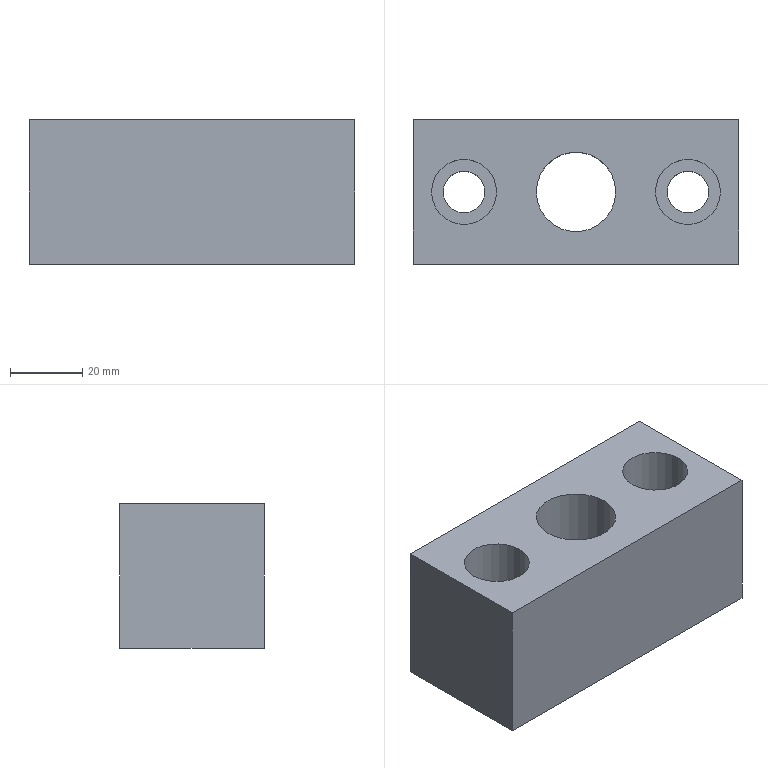Part | STEP file | lll_id4838_x_t | 1 solid | 15 faces | box 90 x 40 x 40 mm | volume 115299 mm3 | plane 9 | cylinder 6 | commonest cylinder face diameters 11.509 x2 18.008 x2 22 x1 30 x1
STEP:
#1=CARTESIAN_POINT('',(2582.,20.,-80.));
#2=VERTEX_POINT('',#1);
#3=CARTESIAN_POINT('',(2582.,-20.,-80.));
#4=VERTEX_POINT('',#3);
#5=CARTESIAN_POINT('',(2582.,10.,-80.));
#6=DIRECTION('',(0.,-1.,0.));
#7=VECTOR('',#6,1.);
#8=LINE('',#5,#7);
#9=EDGE_CURVE('',#2,#4,#8,.T.);
#10=ORIENTED_EDGE('',*,*,#9,.F.);
#11=CARTESIAN_POINT('',(2672.,20.,-80.));
#12=VERTEX_POINT('',#11);
#13=CARTESIAN_POINT('',(2632.,20.,-80.));
#14=DIRECTION('',(-1.,0.,0.));
#15=VECTOR('',#14,1.);
#16=LINE('',#13,#15);
#17=EDGE_CURVE('',#12,#2,#16,.T.);
#18=ORIENTED_EDGE('',*,*,#17,.F.);
#19=CARTESIAN_POINT('',(2672.,-20.,-80.));
#20=VERTEX_POINT('',#19);
#21=CARTESIAN_POINT('',(2672.,10.,-80.));
#22=DIRECTION('',(0.,1.,0.));
#23=VECTOR('',#22,1.);
#24=LINE('',#21,#23);
#25=EDGE_CURVE('',#20,#12,#24,.T.);
#26=ORIENTED_EDGE('',*,*,#25,.F.);
#27=CARTESIAN_POINT('',(2632.,-20.,-80.));
#28=DIRECTION('',(1.,0.,0.));
#29=VECTOR('',#28,1.);
#30=LINE('',#27,#29);
#31=EDGE_CURVE('',#4,#20,#30,.T.);
#32=ORIENTED_EDGE('',*,*,#31,.F.);
#33=EDGE_LOOP('',(#10,#18,#26,#32));
#34=FACE_BOUND('',#33,.T.);
#35=CARTESIAN_POINT('',(2663.755,0.00007613,-80.));
#36=VERTEX_POINT('',#35);
#37=CARTESIAN_POINT('',(2658.,0.00007613,-80.));
#38=DIRECTION('',(0.,0.,-1.));
#39=DIRECTION('',(1.,0.,0.));
#40=AXIS2_PLACEMENT_3D('',#37,#38,#39);
#41=CIRCLE('',#40,5.755);
#42=EDGE_CURVE('',#36,#36,#41,.T.);
#43=ORIENTED_EDGE('',*,*,#42,.F.);
#44=EDGE_LOOP('',(#43));
#45=FACE_BOUND('',#44,.T.);
#46=CARTESIAN_POINT('',(2601.755,0.00007613,-80.));
#47=VERTEX_POINT('',#46);
#48=CARTESIAN_POINT('',(2596.,0.00007613,-80.));
#49=DIRECTION('',(0.,0.,-1.));
#50=DIRECTION('',(1.,0.,0.));
#51=AXIS2_PLACEMENT_3D('',#48,#49,#50);
#52=CIRCLE('',#51,5.755);
#53=EDGE_CURVE('',#47,#47,#52,.T.);
#54=ORIENTED_EDGE('',*,*,#53,.F.);
#55=EDGE_LOOP('',(#54));
#56=FACE_BOUND('',#55,.T.);
#57=CARTESIAN_POINT('',(2612.,0.00007613,-80.));
#58=VERTEX_POINT('',#57);
#59=CARTESIAN_POINT('',(2627.,0.00007613,-80.));
#60=DIRECTION('',(0.,0.,1.));
#61=DIRECTION('',(-1.,0.,0.));
#62=AXIS2_PLACEMENT_3D('',#59,#60,#61);
#63=CIRCLE('',#62,15.);
#64=EDGE_CURVE('',#58,#58,#63,.T.);
#65=ORIENTED_EDGE('',*,*,#64,.T.);
#66=EDGE_LOOP('',(#65));
#67=FACE_BOUND('',#66,.T.);
#68=CARTESIAN_POINT('',(2632.,10.,-80.));
#69=DIRECTION('',(0.,0.,-1.));
#70=DIRECTION('',(1.,0.,0.));
#71=AXIS2_PLACEMENT_3D('',#68,#69,#70);
#72=PLANE('',#71);
#73=ADVANCED_FACE('',(#34,#45,#56,#67),#72,.T.);
#74=CARTESIAN_POINT('',(2638.,0.00007613,-40.));
#75=VERTEX_POINT('',#74);
#76=CARTESIAN_POINT('',(2627.,0.00007613,-40.));
#77=DIRECTION('',(0.,0.,1.));
#78=DIRECTION('',(1.,0.,0.));
#79=AXIS2_PLACEMENT_3D('',#76,#77,#78);
#80=CIRCLE('',#79,11.);
#81=EDGE_CURVE('',#75,#75,#80,.T.);
#82=ORIENTED_EDGE('',*,*,#81,.F.);
#83=EDGE_LOOP('',(#82));
#84=FACE_BOUND('',#83,.T.);
#85=CARTESIAN_POINT('',(2648.996,0.00007613,-40.));
#86=VERTEX_POINT('',#85);
#87=CARTESIAN_POINT('',(2658.,0.00007613,-40.));
#88=DIRECTION('',(0.,0.,-1.));
#89=DIRECTION('',(-1.,0.,0.));
#90=AXIS2_PLACEMENT_3D('',#87,#88,#89);
#91=CIRCLE('',#90,9.004);
#92=EDGE_CURVE('',#86,#86,#91,.T.);
#93=ORIENTED_EDGE('',*,*,#92,.T.);
#94=EDGE_LOOP('',(#93));
#95=FACE_BOUND('',#94,.T.);
#96=CARTESIAN_POINT('',(2582.,20.,-40.));
#97=VERTEX_POINT('',#96);
#98=CARTESIAN_POINT('',(2672.,20.,-40.));
#99=VERTEX_POINT('',#98);
#100=CARTESIAN_POINT('',(2632.,20.,-40.));
#101=DIRECTION('',(1.,0.,0.));
#102=VECTOR('',#101,1.);
#103=LINE('',#100,#102);
#104=EDGE_CURVE('',#97,#99,#103,.T.);
#105=ORIENTED_EDGE('',*,*,#104,.F.);
#106=CARTESIAN_POINT('',(2582.,-20.,-40.));
#107=VERTEX_POINT('',#106);
#108=CARTESIAN_POINT('',(2582.,10.,-40.));
#109=DIRECTION('',(0.,1.,0.));
#110=VECTOR('',#109,1.);
#111=LINE('',#108,#110);
#112=EDGE_CURVE('',#107,#97,#111,.T.);
#113=ORIENTED_EDGE('',*,*,#112,.F.);
#114=CARTESIAN_POINT('',(2672.,-20.,-40.));
#115=VERTEX_POINT('',#114);
#116=CARTESIAN_POINT('',(2632.,-20.,-40.));
#117=DIRECTION('',(-1.,0.,0.));
#118=VECTOR('',#117,1.);
#119=LINE('',#116,#118);
#120=EDGE_CURVE('',#115,#107,#119,.T.);
#121=ORIENTED_EDGE('',*,*,#120,.F.);
#122=CARTESIAN_POINT('',(2672.,10.,-40.));
#123=DIRECTION('',(0.,-1.,0.));
#124=VECTOR('',#123,1.);
#125=LINE('',#122,#124);
#126=EDGE_CURVE('',#99,#115,#125,.T.);
#127=ORIENTED_EDGE('',*,*,#126,.F.);
#128=EDGE_LOOP('',(#105,#113,#121,#127));
#129=FACE_BOUND('',#128,.T.);
#130=CARTESIAN_POINT('',(2586.996,0.00007613,-40.));
#131=VERTEX_POINT('',#130);
#132=CARTESIAN_POINT('',(2596.,0.00007613,-40.));
#133=DIRECTION('',(0.,0.,-1.));
#134=DIRECTION('',(-1.,0.,0.));
#135=AXIS2_PLACEMENT_3D('',#132,#133,#134);
#136=CIRCLE('',#135,9.004);
#137=EDGE_CURVE('',#131,#131,#136,.T.);
#138=ORIENTED_EDGE('',*,*,#137,.T.);
#139=EDGE_LOOP('',(#138));
#140=FACE_BOUND('',#139,.T.);
#141=CARTESIAN_POINT('',(2632.,10.,-40.));
#142=DIRECTION('',(0.,0.,1.));
#143=DIRECTION('',(-1.,0.,0.));
#144=AXIS2_PLACEMENT_3D('',#141,#142,#143);
#145=PLANE('',#144);
#146=ADVANCED_FACE('',(#84,#95,#129,#140),#145,.T.);
#147=CARTESIAN_POINT('',(2582.,20.,-80.));
#148=DIRECTION('',(0.,0.,1.));
#149=VECTOR('',#148,1.);
#150=LINE('',#147,#149);
#151=EDGE_CURVE('',#2,#97,#150,.T.);
#152=ORIENTED_EDGE('',*,*,#151,.T.);
#153=ORIENTED_EDGE('',*,*,#104,.T.);
#154=CARTESIAN_POINT('',(2672.,20.,-80.));
#155=DIRECTION('',(0.,0.,1.));
#156=VECTOR('',#155,1.);
#157=LINE('',#154,#156);
#158=EDGE_CURVE('',#12,#99,#157,.T.);
#159=ORIENTED_EDGE('',*,*,#158,.F.);
#160=ORIENTED_EDGE('',*,*,#17,.T.);
#161=EDGE_LOOP('',(#152,#153,#159,#160));
#162=FACE_OUTER_BOUND('',#161,.T.);
#163=CARTESIAN_POINT('',(2632.,20.,-80.));
#164=DIRECTION('',(0.,1.,0.));
#165=DIRECTION('',(0.,0.,-1.));
#166=AXIS2_PLACEMENT_3D('',#163,#164,#165);
#167=PLANE('',#166);
#168=ADVANCED_FACE('',(#162),#167,.T.);
#169=ORIENTED_EDGE('',*,*,#158,.T.);
#170=ORIENTED_EDGE('',*,*,#126,.T.);
#171=CARTESIAN_POINT('',(2672.,-20.,-80.));
#172=DIRECTION('',(0.,0.,1.));
#173=VECTOR('',#172,1.);
#174=LINE('',#171,#173);
#175=EDGE_CURVE('',#20,#115,#174,.T.);
#176=ORIENTED_EDGE('',*,*,#175,.F.);
#177=ORIENTED_EDGE('',*,*,#25,.T.);
#178=EDGE_LOOP('',(#169,#170,#176,#177));
#179=FACE_OUTER_BOUND('',#178,.T.);
#180=CARTESIAN_POINT('',(2672.,10.,-80.));
#181=DIRECTION('',(1.,0.,0.));
#182=DIRECTION('',(0.,0.,1.));
#183=AXIS2_PLACEMENT_3D('',#180,#181,#182);
#184=PLANE('',#183);
#185=ADVANCED_FACE('',(#179),#184,.T.);
#186=ORIENTED_EDGE('',*,*,#175,.T.);
#187=ORIENTED_EDGE('',*,*,#120,.T.);
#188=CARTESIAN_POINT('',(2582.,-20.,-80.));
#189=DIRECTION('',(0.,0.,1.));
#190=VECTOR('',#189,1.);
#191=LINE('',#188,#190);
#192=EDGE_CURVE('',#4,#107,#191,.T.);
#193=ORIENTED_EDGE('',*,*,#192,.F.);
#194=ORIENTED_EDGE('',*,*,#31,.T.);
#195=EDGE_LOOP('',(#186,#187,#193,#194));
#196=FACE_OUTER_BOUND('',#195,.T.);
#197=CARTESIAN_POINT('',(2632.,-20.,-80.));
#198=DIRECTION('',(0.,-1.,0.));
#199=DIRECTION('',(0.,0.,1.));
#200=AXIS2_PLACEMENT_3D('',#197,#198,#199);
#201=PLANE('',#200);
#202=ADVANCED_FACE('',(#196),#201,.T.);
#203=ORIENTED_EDGE('',*,*,#9,.T.);
#204=ORIENTED_EDGE('',*,*,#192,.T.);
#205=ORIENTED_EDGE('',*,*,#112,.T.);
#206=ORIENTED_EDGE('',*,*,#151,.F.);
#207=EDGE_LOOP('',(#203,#204,#205,#206));
#208=FACE_OUTER_BOUND('',#207,.T.);
#209=CARTESIAN_POINT('',(2582.,10.,-80.));
#210=DIRECTION('',(-1.,0.,0.));
#211=DIRECTION('',(0.,0.,-1.));
#212=AXIS2_PLACEMENT_3D('',#209,#210,#211);
#213=PLANE('',#212);
#214=ADVANCED_FACE('',(#208),#213,.T.);
#215=ORIENTED_EDGE('',*,*,#42,.T.);
#216=EDGE_LOOP('',(#215));
#217=FACE_BOUND('',#216,.T.);
#218=CARTESIAN_POINT('',(2663.755,0.00007613,-55.));
#219=VERTEX_POINT('',#218);
#220=CARTESIAN_POINT('',(2658.,0.00007613,-55.));
#221=DIRECTION('',(0.,0.,-1.));
#222=DIRECTION('',(1.,0.,0.));
#223=AXIS2_PLACEMENT_3D('',#220,#221,#222);
#224=CIRCLE('',#223,5.755);
#225=EDGE_CURVE('',#219,#219,#224,.T.);
#226=ORIENTED_EDGE('',*,*,#225,.F.);
#227=EDGE_LOOP('',(#226));
#228=FACE_BOUND('',#227,.T.);
#229=CARTESIAN_POINT('',(2658.,0.00007613,-33.));
#230=DIRECTION('',(0.,0.,-1.));
#231=DIRECTION('',(-1.,0.,0.));
#232=AXIS2_PLACEMENT_3D('',#229,#230,#231);
#233=CYLINDRICAL_SURFACE('',#232,5.755);
#234=ADVANCED_FACE('',(#217,#228),#233,.F.);
#235=ORIENTED_EDGE('',*,*,#225,.T.);
#236=EDGE_LOOP('',(#235));
#237=FACE_BOUND('',#236,.T.);
#238=CARTESIAN_POINT('',(2648.996,0.00007613,-55.));
#239=VERTEX_POINT('',#238);
#240=CARTESIAN_POINT('',(2658.,0.00007613,-55.));
#241=DIRECTION('',(0.,0.,-1.));
#242=DIRECTION('',(-1.,0.,0.));
#243=AXIS2_PLACEMENT_3D('',#240,#241,#242);
#244=CIRCLE('',#243,9.004);
#245=EDGE_CURVE('',#239,#239,#244,.T.);
#246=ORIENTED_EDGE('',*,*,#245,.F.);
#247=EDGE_LOOP('',(#246));
#248=FACE_BOUND('',#247,.T.);
#249=CARTESIAN_POINT('',(2658.,0.00007613,-55.));
#250=DIRECTION('',(0.,0.,-1.));
#251=DIRECTION('',(1.,0.,0.));
#252=AXIS2_PLACEMENT_3D('',#249,#250,#251);
#253=PLANE('',#252);
#254=ADVANCED_FACE('',(#237,#248),#253,.F.);
#255=ORIENTED_EDGE('',*,*,#245,.T.);
#256=EDGE_LOOP('',(#255));
#257=FACE_BOUND('',#256,.T.);
#258=ORIENTED_EDGE('',*,*,#92,.F.);
#259=EDGE_LOOP('',(#258));
#260=FACE_BOUND('',#259,.T.);
#261=CARTESIAN_POINT('',(2658.,0.00007613,-40.));
#262=DIRECTION('',(0.,0.,-1.));
#263=DIRECTION('',(-1.,0.,0.));
#264=AXIS2_PLACEMENT_3D('',#261,#262,#263);
#265=CYLINDRICAL_SURFACE('',#264,9.004);
#266=ADVANCED_FACE('',(#257,#260),#265,.F.);
#267=ORIENTED_EDGE('',*,*,#53,.T.);
#268=EDGE_LOOP('',(#267));
#269=FACE_BOUND('',#268,.T.);
#270=CARTESIAN_POINT('',(2601.755,0.00007613,-55.));
#271=VERTEX_POINT('',#270);
#272=CARTESIAN_POINT('',(2596.,0.00007613,-55.));
#273=DIRECTION('',(0.,0.,-1.));
#274=DIRECTION('',(1.,0.,0.));
#275=AXIS2_PLACEMENT_3D('',#272,#273,#274);
#276=CIRCLE('',#275,5.755);
#277=EDGE_CURVE('',#271,#271,#276,.T.);
#278=ORIENTED_EDGE('',*,*,#277,.F.);
#279=EDGE_LOOP('',(#278));
#280=FACE_BOUND('',#279,.T.);
#281=CARTESIAN_POINT('',(2596.,0.00007613,-33.));
#282=DIRECTION('',(0.,0.,-1.));
#283=DIRECTION('',(-1.,0.,0.));
#284=AXIS2_PLACEMENT_3D('',#281,#282,#283);
#285=CYLINDRICAL_SURFACE('',#284,5.755);
#286=ADVANCED_FACE('',(#269,#280),#285,.F.);
#287=ORIENTED_EDGE('',*,*,#277,.T.);
#288=EDGE_LOOP('',(#287));
#289=FACE_BOUND('',#288,.T.);
#290=CARTESIAN_POINT('',(2586.996,0.00007613,-55.));
#291=VERTEX_POINT('',#290);
#292=CARTESIAN_POINT('',(2596.,0.00007613,-55.));
#293=DIRECTION('',(0.,0.,-1.));
#294=DIRECTION('',(-1.,0.,0.));
#295=AXIS2_PLACEMENT_3D('',#292,#293,#294);
#296=CIRCLE('',#295,9.004);
#297=EDGE_CURVE('',#291,#291,#296,.T.);
#298=ORIENTED_EDGE('',*,*,#297,.F.);
#299=EDGE_LOOP('',(#298));
#300=FACE_BOUND('',#299,.T.);
#301=CARTESIAN_POINT('',(2596.,0.00007613,-55.));
#302=DIRECTION('',(0.,0.,-1.));
#303=DIRECTION('',(1.,0.,0.));
#304=AXIS2_PLACEMENT_3D('',#301,#302,#303);
#305=PLANE('',#304);
#306=ADVANCED_FACE('',(#289,#300),#305,.F.);
#307=ORIENTED_EDGE('',*,*,#297,.T.);
#308=EDGE_LOOP('',(#307));
#309=FACE_BOUND('',#308,.T.);
#310=ORIENTED_EDGE('',*,*,#137,.F.);
#311=EDGE_LOOP('',(#310));
#312=FACE_BOUND('',#311,.T.);
#313=CARTESIAN_POINT('',(2596.,0.00007613,-40.));
#314=DIRECTION('',(0.,0.,-1.));
#315=DIRECTION('',(-1.,0.,0.));
#316=AXIS2_PLACEMENT_3D('',#313,#314,#315);
#317=CYLINDRICAL_SURFACE('',#316,9.004);
#318=ADVANCED_FACE('',(#309,#312),#317,.F.);
#319=ORIENTED_EDGE('',*,*,#64,.F.);
#320=EDGE_LOOP('',(#319));
#321=FACE_BOUND('',#320,.T.);
#322=CARTESIAN_POINT('',(2642.,0.00007613,-78.));
#323=VERTEX_POINT('',#322);
#324=CARTESIAN_POINT('',(2627.,0.00007613,-78.));
#325=DIRECTION('',(0.,0.,-1.));
#326=DIRECTION('',(1.,0.,0.));
#327=AXIS2_PLACEMENT_3D('',#324,#325,#326);
#328=CIRCLE('',#327,15.);
#329=EDGE_CURVE('',#323,#323,#328,.T.);
#330=ORIENTED_EDGE('',*,*,#329,.F.);
#331=EDGE_LOOP('',(#330));
#332=FACE_BOUND('',#331,.T.);
#333=CARTESIAN_POINT('',(2627.,0.00007613,-78.));
#334=DIRECTION('',(0.,0.,-1.));
#335=DIRECTION('',(-1.,0.,0.));
#336=AXIS2_PLACEMENT_3D('',#333,#334,#335);
#337=CYLINDRICAL_SURFACE('',#336,15.);
#338=ADVANCED_FACE('',(#321,#332),#337,.F.);
#339=CARTESIAN_POINT('',(2638.,0.00007613,-78.));
#340=VERTEX_POINT('',#339);
#341=CARTESIAN_POINT('',(2627.,0.00007613,-78.));
#342=DIRECTION('',(0.,0.,1.));
#343=DIRECTION('',(1.,0.,0.));
#344=AXIS2_PLACEMENT_3D('',#341,#342,#343);
#345=CIRCLE('',#344,11.);
#346=EDGE_CURVE('',#340,#340,#345,.T.);
#347=ORIENTED_EDGE('',*,*,#346,.T.);
#348=EDGE_LOOP('',(#347));
#349=FACE_BOUND('',#348,.T.);
#350=ORIENTED_EDGE('',*,*,#329,.T.);
#351=EDGE_LOOP('',(#350));
#352=FACE_BOUND('',#351,.T.);
#353=CARTESIAN_POINT('',(2627.,0.00007613,-78.));
#354=DIRECTION('',(0.,0.,1.));
#355=DIRECTION('',(1.,0.,0.));
#356=AXIS2_PLACEMENT_3D('',#353,#354,#355);
#357=PLANE('',#356);
#358=ADVANCED_FACE('',(#349,#352),#357,.F.);
#359=ORIENTED_EDGE('',*,*,#81,.T.);
#360=EDGE_LOOP('',(#359));
#361=FACE_BOUND('',#360,.T.);
#362=ORIENTED_EDGE('',*,*,#346,.F.);
#363=EDGE_LOOP('',(#362));
#364=FACE_BOUND('',#363,.T.);
#365=CARTESIAN_POINT('',(2627.,0.00007613,-142.));
#366=DIRECTION('',(0.,0.,1.));
#367=DIRECTION('',(1.,0.,0.));
#368=AXIS2_PLACEMENT_3D('',#365,#366,#367);
#369=CYLINDRICAL_SURFACE('',#368,11.);
#370=ADVANCED_FACE('',(#361,#364),#369,.F.);
#371=CLOSED_SHELL('',(#73,#146,#168,#185,#202,#214,#234,#254,#266,#286,#306,#318,#338,#358,#370));
#372=MANIFOLD_SOLID_BREP('',#371);
#373=(LENGTH_UNIT()NAMED_UNIT(*)SI_UNIT(.MILLI.,.METRE.));
#374=UNCERTAINTY_MEASURE_WITH_UNIT(LENGTH_MEASURE(0.00002),#373,'','');
#375=(NAMED_UNIT(*)PLANE_ANGLE_UNIT()SI_UNIT($,.RADIAN.));
#376=PLANE_ANGLE_MEASURE_WITH_UNIT(PLANE_ANGLE_MEASURE(0.01745),#375);
#377=DIMENSIONAL_EXPONENTS(0.,0.,0.,0.,0.,0.,0.);
#378=(CONVERSION_BASED_UNIT('DEGREE',#376)NAMED_UNIT(#377)PLANE_ANGLE_UNIT());
#379=(NAMED_UNIT(*)SI_UNIT($,.STERADIAN.)SOLID_ANGLE_UNIT());
#380=(GEOMETRIC_REPRESENTATION_CONTEXT(3)GLOBAL_UNCERTAINTY_ASSIGNED_CONTEXT((#374))GLOBAL_UNIT_ASSIGNED_CONTEXT((#373,#378,#379))REPRESENTATION_CONTEXT('',''));
#381=ADVANCED_BREP_SHAPE_REPRESENTATION('',(#372),#380);